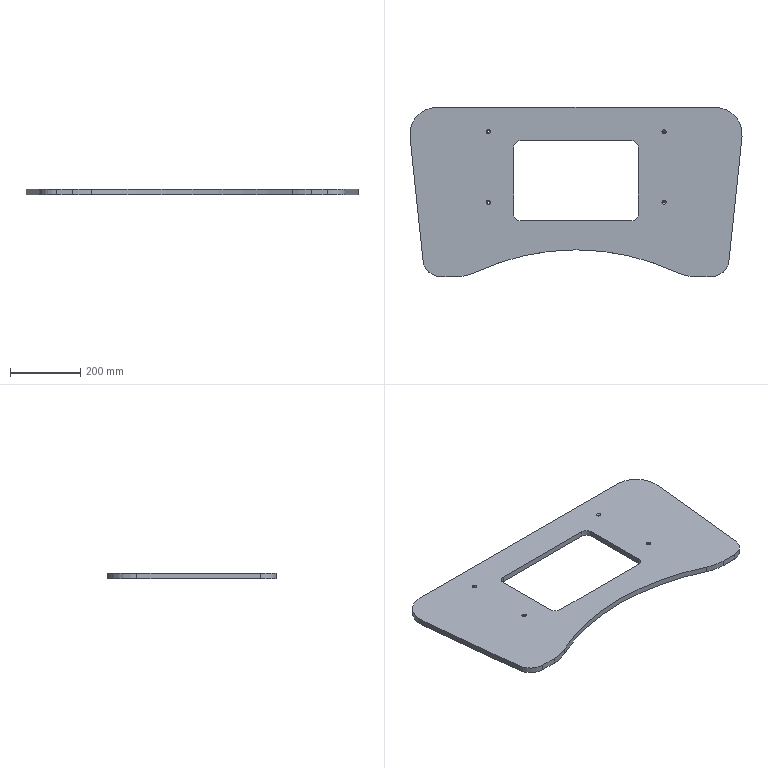Part | NX | features BREP 1 | 1 solid | 38 faces | box 948.321 x 482.727 x 15.875 mm | volume 5145279 mm3 | cylinder 19 | plane 11 | cone 8 | commonest cylinder face diameters 6.604 x8 38.1 x4 101.6 x2 152.4 x2 254 x2 1347 x1
STEP:
#1=CARTESIAN_POINT('',(-386.065,-482.727,0.));
#2=VERTEX_POINT('',#1);
#3=CARTESIAN_POINT('',(-340.836,-482.727,0.));
#4=VERTEX_POINT('',#3);
#5=CARTESIAN_POINT('',(-386.065,-482.727,0.));
#6=DIRECTION('',(1.,0.,0.));
#7=VECTOR('',#6,1000.);
#8=LINE('',#5,#7);
#9=EDGE_CURVE('',#2,#4,#8,.T.);
#10=ORIENTED_EDGE('',*,*,#9,.F.);
#11=CARTESIAN_POINT('',(-436.586,-437.244,0.));
#12=VERTEX_POINT('',#11);
#13=CARTESIAN_POINT('',(-386.065,-431.927,0.));
#14=DIRECTION('',(0.,0.,-1.));
#15=DIRECTION('',(0.,-1.,0.));
#16=AXIS2_PLACEMENT_3D('',#13,#14,#15);
#17=CIRCLE('',#16,50.8);
#18=EDGE_CURVE('',#2,#12,#17,.T.);
#19=ORIENTED_EDGE('',*,*,#18,.T.);
#20=CARTESIAN_POINT('',(-473.742,-84.175,0.));
#21=VERTEX_POINT('',#20);
#22=CARTESIAN_POINT('',(-473.742,-84.175,0.));
#23=DIRECTION('',(0.1047,-0.9945,0.));
#24=VECTOR('',#23,1000.);
#25=LINE('',#22,#24);
#26=EDGE_CURVE('',#21,#12,#25,.T.);
#27=ORIENTED_EDGE('',*,*,#26,.F.);
#28=CARTESIAN_POINT('',(-397.96,0.,0.));
#29=VERTEX_POINT('',#28);
#30=CARTESIAN_POINT('',(-397.96,-76.2,0.));
#31=DIRECTION('',(0.,0.,-1.));
#32=DIRECTION('',(-0.9945,-0.1047,0.));
#33=AXIS2_PLACEMENT_3D('',#30,#31,#32);
#34=CIRCLE('',#33,76.2);
#35=EDGE_CURVE('',#21,#29,#34,.T.);
#36=ORIENTED_EDGE('',*,*,#35,.T.);
#37=CARTESIAN_POINT('',(397.96,0.,0.));
#38=VERTEX_POINT('',#37);
#39=CARTESIAN_POINT('',(397.96,0.,0.));
#40=DIRECTION('',(-1.,0.,0.));
#41=VECTOR('',#40,1000.);
#42=LINE('',#39,#41);
#43=EDGE_CURVE('',#38,#29,#42,.T.);
#44=ORIENTED_EDGE('',*,*,#43,.F.);
#45=CARTESIAN_POINT('',(473.742,-84.175,0.));
#46=VERTEX_POINT('',#45);
#47=CARTESIAN_POINT('',(397.96,-76.2,0.));
#48=DIRECTION('',(0.,0.,-1.));
#49=DIRECTION('',(0.,1.,0.));
#50=AXIS2_PLACEMENT_3D('',#47,#48,#49);
#51=CIRCLE('',#50,76.2);
#52=EDGE_CURVE('',#38,#46,#51,.T.);
#53=ORIENTED_EDGE('',*,*,#52,.T.);
#54=CARTESIAN_POINT('',(436.586,-437.244,0.));
#55=VERTEX_POINT('',#54);
#56=CARTESIAN_POINT('',(436.586,-437.244,0.));
#57=DIRECTION('',(0.1047,0.9945,0.));
#58=VECTOR('',#57,1000.);
#59=LINE('',#56,#58);
#60=EDGE_CURVE('',#55,#46,#59,.T.);
#61=ORIENTED_EDGE('',*,*,#60,.F.);
#62=CARTESIAN_POINT('',(386.065,-482.727,0.));
#63=VERTEX_POINT('',#62);
#64=CARTESIAN_POINT('',(386.065,-431.927,0.));
#65=DIRECTION('',(0.,0.,-1.));
#66=DIRECTION('',(0.9945,-0.1047,0.));
#67=AXIS2_PLACEMENT_3D('',#64,#65,#66);
#68=CIRCLE('',#67,50.8);
#69=EDGE_CURVE('',#55,#63,#68,.T.);
#70=ORIENTED_EDGE('',*,*,#69,.T.);
#71=CARTESIAN_POINT('',(340.836,-482.727,0.));
#72=VERTEX_POINT('',#71);
#73=CARTESIAN_POINT('',(340.836,-482.727,0.));
#74=DIRECTION('',(1.,0.,0.));
#75=VECTOR('',#74,1000.);
#76=LINE('',#73,#75);
#77=EDGE_CURVE('',#72,#63,#76,.T.);
#78=ORIENTED_EDGE('',*,*,#77,.F.);
#79=CARTESIAN_POINT('',(286.753,-470.636,0.));
#80=VERTEX_POINT('',#79);
#81=CARTESIAN_POINT('',(340.836,-355.727,0.));
#82=DIRECTION('',(0.,0.,-1.));
#83=DIRECTION('',(0.,-1.,0.));
#84=AXIS2_PLACEMENT_3D('',#81,#82,#83);
#85=CIRCLE('',#84,127.);
#86=EDGE_CURVE('',#72,#80,#85,.T.);
#87=ORIENTED_EDGE('',*,*,#86,.T.);
#88=CARTESIAN_POINT('',(-286.753,-470.636,0.));
#89=VERTEX_POINT('',#88);
#90=CARTESIAN_POINT('',(0.,-1079.892,0.));
#91=DIRECTION('',(0.,0.,1.));
#92=DIRECTION('',(0.4259,0.9048,0.));
#93=AXIS2_PLACEMENT_3D('',#90,#91,#92);
#94=CIRCLE('',#93,673.365);
#95=EDGE_CURVE('',#80,#89,#94,.T.);
#96=ORIENTED_EDGE('',*,*,#95,.T.);
#97=CARTESIAN_POINT('',(-340.836,-355.727,0.));
#98=DIRECTION('',(0.,0.,-1.));
#99=DIRECTION('',(0.4259,-0.9048,0.));
#100=AXIS2_PLACEMENT_3D('',#97,#98,#99);
#101=CIRCLE('',#100,127.);
#102=EDGE_CURVE('',#89,#4,#101,.T.);
#103=ORIENTED_EDGE('',*,*,#102,.T.);
#104=EDGE_LOOP('',(#10,#19,#27,#36,#44,#53,#61,#70,#78,#87,#96,#103));
#105=FACE_BOUND('',#104,.T.);
#106=CARTESIAN_POINT('',(-246.888,-270.51,0.));
#107=VERTEX_POINT('',#106);
#108=CARTESIAN_POINT('',(-253.492,-270.51,0.));
#109=VERTEX_POINT('',#108);
#110=CARTESIAN_POINT('',(-250.19,-270.51,0.));
#111=DIRECTION('',(0.,0.,1.));
#112=DIRECTION('',(1.,0.,0.));
#113=AXIS2_PLACEMENT_3D('',#110,#111,#112);
#114=CIRCLE('',#113,3.302);
#115=EDGE_CURVE('',#107,#109,#114,.T.);
#116=ORIENTED_EDGE('',*,*,#115,.T.);
#117=CARTESIAN_POINT('',(-250.19,-270.51,0.));
#118=DIRECTION('',(0.,0.,1.));
#119=DIRECTION('',(-1.,0.,0.));
#120=AXIS2_PLACEMENT_3D('',#117,#118,#119);
#121=CIRCLE('',#120,3.302);
#122=EDGE_CURVE('',#109,#107,#121,.T.);
#123=ORIENTED_EDGE('',*,*,#122,.T.);
#124=EDGE_LOOP('',(#116,#123));
#125=FACE_BOUND('',#124,.T.);
#126=CARTESIAN_POINT('',(254.762,-69.85,0.));
#127=VERTEX_POINT('',#126);
#128=CARTESIAN_POINT('',(248.158,-69.85,0.));
#129=VERTEX_POINT('',#128);
#130=CARTESIAN_POINT('',(251.46,-69.85,0.));
#131=DIRECTION('',(0.,0.,1.));
#132=DIRECTION('',(1.,0.,0.));
#133=AXIS2_PLACEMENT_3D('',#130,#131,#132);
#134=CIRCLE('',#133,3.302);
#135=EDGE_CURVE('',#127,#129,#134,.T.);
#136=ORIENTED_EDGE('',*,*,#135,.T.);
#137=CARTESIAN_POINT('',(251.46,-69.85,0.));
#138=DIRECTION('',(0.,0.,1.));
#139=DIRECTION('',(-1.,0.,0.));
#140=AXIS2_PLACEMENT_3D('',#137,#138,#139);
#141=CIRCLE('',#140,3.302);
#142=EDGE_CURVE('',#129,#127,#141,.T.);
#143=ORIENTED_EDGE('',*,*,#142,.T.);
#144=EDGE_LOOP('',(#136,#143));
#145=FACE_BOUND('',#144,.T.);
#146=CARTESIAN_POINT('',(-177.8,-304.8,0.));
#147=VERTEX_POINT('',#146);
#148=CARTESIAN_POINT('',(-158.75,-323.85,0.));
#149=VERTEX_POINT('',#148);
#150=CARTESIAN_POINT('',(-158.75,-304.8,0.));
#151=DIRECTION('',(0.,0.,1.));
#152=DIRECTION('',(-1.,0.,0.));
#153=AXIS2_PLACEMENT_3D('',#150,#151,#152);
#154=CIRCLE('',#153,19.05);
#155=EDGE_CURVE('',#147,#149,#154,.T.);
#156=ORIENTED_EDGE('',*,*,#155,.T.);
#157=CARTESIAN_POINT('',(158.75,-323.85,0.));
#158=VERTEX_POINT('',#157);
#159=CARTESIAN_POINT('',(-158.75,-323.85,0.));
#160=DIRECTION('',(1.,0.,0.));
#161=VECTOR('',#160,1000.);
#162=LINE('',#159,#161);
#163=EDGE_CURVE('',#149,#158,#162,.T.);
#164=ORIENTED_EDGE('',*,*,#163,.T.);
#165=CARTESIAN_POINT('',(177.8,-304.8,0.));
#166=VERTEX_POINT('',#165);
#167=CARTESIAN_POINT('',(158.75,-304.8,0.));
#168=DIRECTION('',(0.,0.,1.));
#169=DIRECTION('',(0.,-1.,0.));
#170=AXIS2_PLACEMENT_3D('',#167,#168,#169);
#171=CIRCLE('',#170,19.05);
#172=EDGE_CURVE('',#158,#166,#171,.T.);
#173=ORIENTED_EDGE('',*,*,#172,.T.);
#174=CARTESIAN_POINT('',(177.8,-114.3,0.));
#175=VERTEX_POINT('',#174);
#176=CARTESIAN_POINT('',(177.8,-304.8,0.));
#177=DIRECTION('',(0.,1.,0.));
#178=VECTOR('',#177,1000.);
#179=LINE('',#176,#178);
#180=EDGE_CURVE('',#166,#175,#179,.T.);
#181=ORIENTED_EDGE('',*,*,#180,.T.);
#182=CARTESIAN_POINT('',(158.75,-95.25,0.));
#183=VERTEX_POINT('',#182);
#184=CARTESIAN_POINT('',(158.75,-114.3,0.));
#185=DIRECTION('',(0.,0.,1.));
#186=DIRECTION('',(1.,0.,0.));
#187=AXIS2_PLACEMENT_3D('',#184,#185,#186);
#188=CIRCLE('',#187,19.05);
#189=EDGE_CURVE('',#175,#183,#188,.T.);
#190=ORIENTED_EDGE('',*,*,#189,.T.);
#191=CARTESIAN_POINT('',(-158.75,-95.25,0.));
#192=VERTEX_POINT('',#191);
#193=CARTESIAN_POINT('',(158.75,-95.25,0.));
#194=DIRECTION('',(-1.,0.,0.));
#195=VECTOR('',#194,1000.);
#196=LINE('',#193,#195);
#197=EDGE_CURVE('',#183,#192,#196,.T.);
#198=ORIENTED_EDGE('',*,*,#197,.T.);
#199=CARTESIAN_POINT('',(-177.8,-114.3,0.));
#200=VERTEX_POINT('',#199);
#201=CARTESIAN_POINT('',(-158.75,-114.3,0.));
#202=DIRECTION('',(0.,0.,1.));
#203=DIRECTION('',(0.,1.,0.));
#204=AXIS2_PLACEMENT_3D('',#201,#202,#203);
#205=CIRCLE('',#204,19.05);
#206=EDGE_CURVE('',#192,#200,#205,.T.);
#207=ORIENTED_EDGE('',*,*,#206,.T.);
#208=CARTESIAN_POINT('',(-177.8,-114.3,0.));
#209=DIRECTION('',(0.,-1.,0.));
#210=VECTOR('',#209,1000.);
#211=LINE('',#208,#210);
#212=EDGE_CURVE('',#200,#147,#211,.T.);
#213=ORIENTED_EDGE('',*,*,#212,.T.);
#214=EDGE_LOOP('',(#156,#164,#173,#181,#190,#198,#207,#213));
#215=FACE_BOUND('',#214,.T.);
#216=CARTESIAN_POINT('',(254.762,-270.51,0.));
#217=VERTEX_POINT('',#216);
#218=CARTESIAN_POINT('',(248.158,-270.51,0.));
#219=VERTEX_POINT('',#218);
#220=CARTESIAN_POINT('',(251.46,-270.51,0.));
#221=DIRECTION('',(0.,0.,1.));
#222=DIRECTION('',(1.,0.,0.));
#223=AXIS2_PLACEMENT_3D('',#220,#221,#222);
#224=CIRCLE('',#223,3.302);
#225=EDGE_CURVE('',#217,#219,#224,.T.);
#226=ORIENTED_EDGE('',*,*,#225,.T.);
#227=CARTESIAN_POINT('',(251.46,-270.51,0.));
#228=DIRECTION('',(0.,0.,1.));
#229=DIRECTION('',(-1.,0.,0.));
#230=AXIS2_PLACEMENT_3D('',#227,#228,#229);
#231=CIRCLE('',#230,3.302);
#232=EDGE_CURVE('',#219,#217,#231,.T.);
#233=ORIENTED_EDGE('',*,*,#232,.T.);
#234=EDGE_LOOP('',(#226,#233));
#235=FACE_BOUND('',#234,.T.);
#236=CARTESIAN_POINT('',(-246.888,-69.85,0.));
#237=VERTEX_POINT('',#236);
#238=CARTESIAN_POINT('',(-253.492,-69.85,0.));
#239=VERTEX_POINT('',#238);
#240=CARTESIAN_POINT('',(-250.19,-69.85,0.));
#241=DIRECTION('',(0.,0.,1.));
#242=DIRECTION('',(1.,0.,0.));
#243=AXIS2_PLACEMENT_3D('',#240,#241,#242);
#244=CIRCLE('',#243,3.302);
#245=EDGE_CURVE('',#237,#239,#244,.T.);
#246=ORIENTED_EDGE('',*,*,#245,.T.);
#247=CARTESIAN_POINT('',(-250.19,-69.85,0.));
#248=DIRECTION('',(0.,0.,1.));
#249=DIRECTION('',(-1.,0.,0.));
#250=AXIS2_PLACEMENT_3D('',#247,#248,#249);
#251=CIRCLE('',#250,3.302);
#252=EDGE_CURVE('',#239,#237,#251,.T.);
#253=ORIENTED_EDGE('',*,*,#252,.T.);
#254=EDGE_LOOP('',(#246,#253));
#255=FACE_BOUND('',#254,.T.);
#256=CARTESIAN_POINT('',(0.,0.,0.));
#257=DIRECTION('',(0.,0.,1.));
#258=DIRECTION('',(1.,0.,0.));
#259=AXIS2_PLACEMENT_3D('',#256,#257,#258);
#260=PLANE('',#259);
#261=ADVANCED_FACE('',(#105,#125,#145,#215,#235,#255),#260,.F.);
#262=CARTESIAN_POINT('',(248.158,-270.51,12.734));
#263=VERTEX_POINT('',#262);
#264=CARTESIAN_POINT('',(248.158,-270.51,0.));
#265=DIRECTION('',(0.,0.,1.));
#266=VECTOR('',#265,1000.);
#267=LINE('',#264,#266);
#268=EDGE_CURVE('',#219,#263,#267,.T.);
#269=ORIENTED_EDGE('',*,*,#268,.T.);
#270=CARTESIAN_POINT('',(254.762,-270.51,12.734));
#271=VERTEX_POINT('',#270);
#272=CARTESIAN_POINT('',(251.46,-270.51,12.734));
#273=DIRECTION('',(0.,0.,1.));
#274=DIRECTION('',(-1.,0.,0.));
#275=AXIS2_PLACEMENT_3D('',#272,#273,#274);
#276=CIRCLE('',#275,3.302);
#277=EDGE_CURVE('',#263,#271,#276,.T.);
#278=ORIENTED_EDGE('',*,*,#277,.T.);
#279=CARTESIAN_POINT('',(254.762,-270.51,0.));
#280=DIRECTION('',(0.,0.,1.));
#281=VECTOR('',#280,1000.);
#282=LINE('',#279,#281);
#283=EDGE_CURVE('',#217,#271,#282,.T.);
#284=ORIENTED_EDGE('',*,*,#283,.F.);
#285=ORIENTED_EDGE('',*,*,#232,.F.);
#286=EDGE_LOOP('',(#269,#278,#284,#285));
#287=FACE_BOUND('',#286,.T.);
#288=CARTESIAN_POINT('',(251.46,-270.51,-4.128));
#289=DIRECTION('',(0.,0.,1.));
#290=DIRECTION('',(-1.,0.,0.));
#291=AXIS2_PLACEMENT_3D('',#288,#289,#290);
#292=CYLINDRICAL_SURFACE('',#291,3.302);
#293=ADVANCED_FACE('',(#287),#292,.F.);
#294=ORIENTED_EDGE('',*,*,#283,.T.);
#295=CARTESIAN_POINT('',(251.46,-270.51,12.734));
#296=DIRECTION('',(0.,0.,-1.));
#297=DIRECTION('',(-1.,0.,0.));
#298=AXIS2_PLACEMENT_3D('',#295,#296,#297);
#299=CIRCLE('',#298,3.302);
#300=EDGE_CURVE('',#263,#271,#299,.T.);
#301=ORIENTED_EDGE('',*,*,#300,.F.);
#302=ORIENTED_EDGE('',*,*,#268,.F.);
#303=ORIENTED_EDGE('',*,*,#225,.F.);
#304=EDGE_LOOP('',(#294,#301,#302,#303));
#305=FACE_BOUND('',#304,.T.);
#306=CARTESIAN_POINT('',(251.46,-270.51,-4.128));
#307=DIRECTION('',(0.,0.,1.));
#308=DIRECTION('',(-1.,0.,0.));
#309=AXIS2_PLACEMENT_3D('',#306,#307,#308);
#310=CYLINDRICAL_SURFACE('',#309,3.302);
#311=ADVANCED_FACE('',(#305),#310,.F.);
#312=CARTESIAN_POINT('',(245.428,-270.51,15.875));
#313=VERTEX_POINT('',#312);
#314=CARTESIAN_POINT('',(248.158,-270.51,12.734));
#315=DIRECTION('',(-0.6561,0.,0.7547));
#316=VECTOR('',#315,1000.);
#317=LINE('',#314,#316);
#318=EDGE_CURVE('',#263,#313,#317,.T.);
#319=ORIENTED_EDGE('',*,*,#318,.F.);
#320=ORIENTED_EDGE('',*,*,#300,.T.);
#321=CARTESIAN_POINT('',(257.493,-270.51,15.875));
#322=VERTEX_POINT('',#321);
#323=CARTESIAN_POINT('',(254.762,-270.51,12.734));
#324=DIRECTION('',(0.6561,0.,0.7547));
#325=VECTOR('',#324,1000.);
#326=LINE('',#323,#325);
#327=EDGE_CURVE('',#271,#322,#326,.T.);
#328=ORIENTED_EDGE('',*,*,#327,.T.);
#329=CARTESIAN_POINT('',(251.46,-270.51,15.875));
#330=DIRECTION('',(0.,0.,1.));
#331=DIRECTION('',(1.,0.,0.));
#332=AXIS2_PLACEMENT_3D('',#329,#330,#331);
#333=CIRCLE('',#332,6.032);
#334=EDGE_CURVE('',#322,#313,#333,.T.);
#335=ORIENTED_EDGE('',*,*,#334,.T.);
#336=EDGE_LOOP('',(#319,#320,#328,#335));
#337=FACE_BOUND('',#336,.T.);
#338=CARTESIAN_POINT('',(251.46,-270.51,14.304));
#339=DIRECTION('',(0.,0.,1.));
#340=DIRECTION('',(-1.,0.,0.));
#341=AXIS2_PLACEMENT_3D('',#338,#339,#340);
#342=CONICAL_SURFACE('',#341,4.667,0.7156);
#343=ADVANCED_FACE('',(#337),#342,.F.);
#344=CARTESIAN_POINT('',(286.753,-470.636,15.875));
#345=VERTEX_POINT('',#344);
#346=CARTESIAN_POINT('',(-286.753,-470.636,15.875));
#347=VERTEX_POINT('',#346);
#348=CARTESIAN_POINT('',(0.,-1079.892,15.875));
#349=DIRECTION('',(0.,0.,1.));
#350=DIRECTION('',(0.4259,0.9048,0.));
#351=AXIS2_PLACEMENT_3D('',#348,#349,#350);
#352=CIRCLE('',#351,673.365);
#353=EDGE_CURVE('',#345,#347,#352,.T.);
#354=ORIENTED_EDGE('',*,*,#353,.F.);
#355=CARTESIAN_POINT('',(340.836,-482.727,15.875));
#356=VERTEX_POINT('',#355);
#357=CARTESIAN_POINT('',(340.836,-355.727,15.875));
#358=DIRECTION('',(0.,0.,1.));
#359=DIRECTION('',(-0.4259,-0.9048,0.));
#360=AXIS2_PLACEMENT_3D('',#357,#358,#359);
#361=CIRCLE('',#360,127.);
#362=EDGE_CURVE('',#345,#356,#361,.T.);
#363=ORIENTED_EDGE('',*,*,#362,.T.);
#364=CARTESIAN_POINT('',(386.065,-482.727,15.875));
#365=VERTEX_POINT('',#364);
#366=CARTESIAN_POINT('',(340.836,-482.727,15.875));
#367=DIRECTION('',(1.,0.,0.));
#368=VECTOR('',#367,1000.);
#369=LINE('',#366,#368);
#370=EDGE_CURVE('',#356,#365,#369,.T.);
#371=ORIENTED_EDGE('',*,*,#370,.T.);
#372=CARTESIAN_POINT('',(436.586,-437.244,15.875));
#373=VERTEX_POINT('',#372);
#374=CARTESIAN_POINT('',(386.065,-431.927,15.875));
#375=DIRECTION('',(0.,0.,1.));
#376=DIRECTION('',(0.,-1.,0.));
#377=AXIS2_PLACEMENT_3D('',#374,#375,#376);
#378=CIRCLE('',#377,50.8);
#379=EDGE_CURVE('',#365,#373,#378,.T.);
#380=ORIENTED_EDGE('',*,*,#379,.T.);
#381=CARTESIAN_POINT('',(473.742,-84.175,15.875));
#382=VERTEX_POINT('',#381);
#383=CARTESIAN_POINT('',(436.586,-437.244,15.875));
#384=DIRECTION('',(0.1047,0.9945,0.));
#385=VECTOR('',#384,1000.);
#386=LINE('',#383,#385);
#387=EDGE_CURVE('',#373,#382,#386,.T.);
#388=ORIENTED_EDGE('',*,*,#387,.T.);
#389=CARTESIAN_POINT('',(397.96,0.,15.875));
#390=VERTEX_POINT('',#389);
#391=CARTESIAN_POINT('',(397.96,-76.2,15.875));
#392=DIRECTION('',(0.,0.,1.));
#393=DIRECTION('',(0.9945,-0.1047,0.));
#394=AXIS2_PLACEMENT_3D('',#391,#392,#393);
#395=CIRCLE('',#394,76.2);
#396=EDGE_CURVE('',#382,#390,#395,.T.);
#397=ORIENTED_EDGE('',*,*,#396,.T.);
#398=CARTESIAN_POINT('',(-397.96,0.,15.875));
#399=VERTEX_POINT('',#398);
#400=CARTESIAN_POINT('',(397.96,0.,15.875));
#401=DIRECTION('',(-1.,0.,0.));
#402=VECTOR('',#401,1000.);
#403=LINE('',#400,#402);
#404=EDGE_CURVE('',#390,#399,#403,.T.);
#405=ORIENTED_EDGE('',*,*,#404,.T.);
#406=CARTESIAN_POINT('',(-473.742,-84.175,15.875));
#407=VERTEX_POINT('',#406);
#408=CARTESIAN_POINT('',(-397.96,-76.2,15.875));
#409=DIRECTION('',(0.,0.,1.));
#410=DIRECTION('',(0.,1.,0.));
#411=AXIS2_PLACEMENT_3D('',#408,#409,#410);
#412=CIRCLE('',#411,76.2);
#413=EDGE_CURVE('',#399,#407,#412,.T.);
#414=ORIENTED_EDGE('',*,*,#413,.T.);
#415=CARTESIAN_POINT('',(-436.586,-437.244,15.875));
#416=VERTEX_POINT('',#415);
#417=CARTESIAN_POINT('',(-473.742,-84.175,15.875));
#418=DIRECTION('',(0.1047,-0.9945,0.));
#419=VECTOR('',#418,1000.);
#420=LINE('',#417,#419);
#421=EDGE_CURVE('',#407,#416,#420,.T.);
#422=ORIENTED_EDGE('',*,*,#421,.T.);
#423=CARTESIAN_POINT('',(-386.065,-482.727,15.875));
#424=VERTEX_POINT('',#423);
#425=CARTESIAN_POINT('',(-386.065,-431.927,15.875));
#426=DIRECTION('',(0.,0.,1.));
#427=DIRECTION('',(-0.9945,-0.1047,0.));
#428=AXIS2_PLACEMENT_3D('',#425,#426,#427);
#429=CIRCLE('',#428,50.8);
#430=EDGE_CURVE('',#416,#424,#429,.T.);
#431=ORIENTED_EDGE('',*,*,#430,.T.);
#432=CARTESIAN_POINT('',(-340.836,-482.727,15.875));
#433=VERTEX_POINT('',#432);
#434=CARTESIAN_POINT('',(-386.065,-482.727,15.875));
#435=DIRECTION('',(1.,0.,0.));
#436=VECTOR('',#435,1000.);
#437=LINE('',#434,#436);
#438=EDGE_CURVE('',#424,#433,#437,.T.);
#439=ORIENTED_EDGE('',*,*,#438,.T.);
#440=CARTESIAN_POINT('',(-340.836,-355.727,15.875));
#441=DIRECTION('',(0.,0.,1.));
#442=DIRECTION('',(0.,-1.,0.));
#443=AXIS2_PLACEMENT_3D('',#440,#441,#442);
#444=CIRCLE('',#443,127.);
#445=EDGE_CURVE('',#433,#347,#444,.T.);
#446=ORIENTED_EDGE('',*,*,#445,.T.);
#447=EDGE_LOOP('',(#354,#363,#371,#380,#388,#397,#405,#414,#422,#431,#439,#446));
#448=FACE_BOUND('',#447,.T.);
#449=CARTESIAN_POINT('',(-244.157,-270.51,15.875));
#450=VERTEX_POINT('',#449);
#451=CARTESIAN_POINT('',(-256.223,-270.51,15.875));
#452=VERTEX_POINT('',#451);
#453=CARTESIAN_POINT('',(-250.19,-270.51,15.875));
#454=DIRECTION('',(0.,0.,1.));
#455=DIRECTION('',(1.,0.,0.));
#456=AXIS2_PLACEMENT_3D('',#453,#454,#455);
#457=CIRCLE('',#456,6.032);
#458=EDGE_CURVE('',#450,#452,#457,.T.);
#459=ORIENTED_EDGE('',*,*,#458,.F.);
#460=CARTESIAN_POINT('',(-250.19,-270.51,15.875));
#461=DIRECTION('',(0.,0.,1.));
#462=DIRECTION('',(-1.,0.,0.));
#463=AXIS2_PLACEMENT_3D('',#460,#461,#462);
#464=CIRCLE('',#463,6.032);
#465=EDGE_CURVE('',#452,#450,#464,.T.);
#466=ORIENTED_EDGE('',*,*,#465,.F.);
#467=EDGE_LOOP('',(#459,#466));
#468=FACE_BOUND('',#467,.T.);
#469=CARTESIAN_POINT('',(257.493,-69.85,15.875));
#470=VERTEX_POINT('',#469);
#471=CARTESIAN_POINT('',(245.428,-69.85,15.875));
#472=VERTEX_POINT('',#471);
#473=CARTESIAN_POINT('',(251.46,-69.85,15.875));
#474=DIRECTION('',(0.,0.,1.));
#475=DIRECTION('',(1.,0.,0.));
#476=AXIS2_PLACEMENT_3D('',#473,#474,#475);
#477=CIRCLE('',#476,6.032);
#478=EDGE_CURVE('',#470,#472,#477,.T.);
#479=ORIENTED_EDGE('',*,*,#478,.F.);
#480=CARTESIAN_POINT('',(251.46,-69.85,15.875));
#481=DIRECTION('',(0.,0.,1.));
#482=DIRECTION('',(-1.,0.,0.));
#483=AXIS2_PLACEMENT_3D('',#480,#481,#482);
#484=CIRCLE('',#483,6.032);
#485=EDGE_CURVE('',#472,#470,#484,.T.);
#486=ORIENTED_EDGE('',*,*,#485,.F.);
#487=EDGE_LOOP('',(#479,#486));
#488=FACE_BOUND('',#487,.T.);
#489=CARTESIAN_POINT('',(158.75,-95.25,15.875));
#490=VERTEX_POINT('',#489);
#491=CARTESIAN_POINT('',(177.8,-114.3,15.875));
#492=VERTEX_POINT('',#491);
#493=CARTESIAN_POINT('',(158.75,-114.3,15.875));
#494=DIRECTION('',(0.,0.,-1.));
#495=DIRECTION('',(0.,1.,0.));
#496=AXIS2_PLACEMENT_3D('',#493,#494,#495);
#497=CIRCLE('',#496,19.05);
#498=EDGE_CURVE('',#490,#492,#497,.T.);
#499=ORIENTED_EDGE('',*,*,#498,.T.);
#500=CARTESIAN_POINT('',(177.8,-304.8,15.875));
#501=VERTEX_POINT('',#500);
#502=CARTESIAN_POINT('',(177.8,-304.8,15.875));
#503=DIRECTION('',(0.,1.,0.));
#504=VECTOR('',#503,1000.);
#505=LINE('',#502,#504);
#506=EDGE_CURVE('',#501,#492,#505,.T.);
#507=ORIENTED_EDGE('',*,*,#506,.F.);
#508=CARTESIAN_POINT('',(158.75,-323.85,15.875));
#509=VERTEX_POINT('',#508);
#510=CARTESIAN_POINT('',(158.75,-304.8,15.875));
#511=DIRECTION('',(0.,0.,-1.));
#512=DIRECTION('',(1.,0.,0.));
#513=AXIS2_PLACEMENT_3D('',#510,#511,#512);
#514=CIRCLE('',#513,19.05);
#515=EDGE_CURVE('',#501,#509,#514,.T.);
#516=ORIENTED_EDGE('',*,*,#515,.T.);
#517=CARTESIAN_POINT('',(-158.75,-323.85,15.875));
#518=VERTEX_POINT('',#517);
#519=CARTESIAN_POINT('',(-158.75,-323.85,15.875));
#520=DIRECTION('',(1.,0.,0.));
#521=VECTOR('',#520,1000.);
#522=LINE('',#519,#521);
#523=EDGE_CURVE('',#518,#509,#522,.T.);
#524=ORIENTED_EDGE('',*,*,#523,.F.);
#525=CARTESIAN_POINT('',(-177.8,-304.8,15.875));
#526=VERTEX_POINT('',#525);
#527=CARTESIAN_POINT('',(-158.75,-304.8,15.875));
#528=DIRECTION('',(0.,0.,-1.));
#529=DIRECTION('',(0.,-1.,0.));
#530=AXIS2_PLACEMENT_3D('',#527,#528,#529);
#531=CIRCLE('',#530,19.05);
#532=EDGE_CURVE('',#518,#526,#531,.T.);
#533=ORIENTED_EDGE('',*,*,#532,.T.);
#534=CARTESIAN_POINT('',(-177.8,-114.3,15.875));
#535=VERTEX_POINT('',#534);
#536=CARTESIAN_POINT('',(-177.8,-114.3,15.875));
#537=DIRECTION('',(0.,-1.,0.));
#538=VECTOR('',#537,1000.);
#539=LINE('',#536,#538);
#540=EDGE_CURVE('',#535,#526,#539,.T.);
#541=ORIENTED_EDGE('',*,*,#540,.F.);
#542=CARTESIAN_POINT('',(-158.75,-95.25,15.875));
#543=VERTEX_POINT('',#542);
#544=CARTESIAN_POINT('',(-158.75,-114.3,15.875));
#545=DIRECTION('',(0.,0.,-1.));
#546=DIRECTION('',(-1.,0.,0.));
#547=AXIS2_PLACEMENT_3D('',#544,#545,#546);
#548=CIRCLE('',#547,19.05);
#549=EDGE_CURVE('',#535,#543,#548,.T.);
#550=ORIENTED_EDGE('',*,*,#549,.T.);
#551=CARTESIAN_POINT('',(158.75,-95.25,15.875));
#552=DIRECTION('',(-1.,0.,0.));
#553=VECTOR('',#552,1000.);
#554=LINE('',#551,#553);
#555=EDGE_CURVE('',#490,#543,#554,.T.);
#556=ORIENTED_EDGE('',*,*,#555,.F.);
#557=EDGE_LOOP('',(#499,#507,#516,#524,#533,#541,#550,#556));
#558=FACE_BOUND('',#557,.T.);
#559=ORIENTED_EDGE('',*,*,#334,.F.);
#560=CARTESIAN_POINT('',(251.46,-270.51,15.875));
#561=DIRECTION('',(0.,0.,1.));
#562=DIRECTION('',(-1.,0.,0.));
#563=AXIS2_PLACEMENT_3D('',#560,#561,#562);
#564=CIRCLE('',#563,6.032);
#565=EDGE_CURVE('',#313,#322,#564,.T.);
#566=ORIENTED_EDGE('',*,*,#565,.F.);
#567=EDGE_LOOP('',(#559,#566));
#568=FACE_BOUND('',#567,.T.);
#569=CARTESIAN_POINT('',(-244.157,-69.85,15.875));
#570=VERTEX_POINT('',#569);
#571=CARTESIAN_POINT('',(-256.223,-69.85,15.875));
#572=VERTEX_POINT('',#571);
#573=CARTESIAN_POINT('',(-250.19,-69.85,15.875));
#574=DIRECTION('',(0.,0.,1.));
#575=DIRECTION('',(1.,0.,0.));
#576=AXIS2_PLACEMENT_3D('',#573,#574,#575);
#577=CIRCLE('',#576,6.032);
#578=EDGE_CURVE('',#570,#572,#577,.T.);
#579=ORIENTED_EDGE('',*,*,#578,.F.);
#580=CARTESIAN_POINT('',(-250.19,-69.85,15.875));
#581=DIRECTION('',(0.,0.,1.));
#582=DIRECTION('',(-1.,0.,0.));
#583=AXIS2_PLACEMENT_3D('',#580,#581,#582);
#584=CIRCLE('',#583,6.032);
#585=EDGE_CURVE('',#572,#570,#584,.T.);
#586=ORIENTED_EDGE('',*,*,#585,.F.);
#587=EDGE_LOOP('',(#579,#586));
#588=FACE_BOUND('',#587,.T.);
#589=CARTESIAN_POINT('',(0.,0.,15.875));
#590=DIRECTION('',(0.,0.,1.));
#591=DIRECTION('',(1.,0.,0.));
#592=AXIS2_PLACEMENT_3D('',#589,#590,#591);
#593=PLANE('',#592);
#594=ADVANCED_FACE('',(#448,#468,#488,#558,#568,#588),#593,.T.);
#595=ORIENTED_EDGE('',*,*,#327,.F.);
#596=ORIENTED_EDGE('',*,*,#277,.F.);
#597=ORIENTED_EDGE('',*,*,#318,.T.);
#598=ORIENTED_EDGE('',*,*,#565,.T.);
#599=EDGE_LOOP('',(#595,#596,#597,#598));
#600=FACE_BOUND('',#599,.T.);
#601=CARTESIAN_POINT('',(251.46,-270.51,14.304));
#602=DIRECTION('',(0.,0.,1.));
#603=DIRECTION('',(-1.,0.,0.));
#604=AXIS2_PLACEMENT_3D('',#601,#602,#603);
#605=CONICAL_SURFACE('',#604,4.667,0.7156);
#606=ADVANCED_FACE('',(#600),#605,.F.);
#607=CARTESIAN_POINT('',(-246.888,-270.51,12.734));
#608=VERTEX_POINT('',#607);
#609=CARTESIAN_POINT('',(-246.888,-270.51,12.734));
#610=DIRECTION('',(0.6561,0.,0.7547));
#611=VECTOR('',#610,1000.);
#612=LINE('',#609,#611);
#613=EDGE_CURVE('',#450,#608,#612,.F.);
#614=ORIENTED_EDGE('',*,*,#613,.T.);
#615=CARTESIAN_POINT('',(-253.492,-270.51,12.734));
#616=VERTEX_POINT('',#615);
#617=CARTESIAN_POINT('',(-250.19,-270.51,12.734));
#618=DIRECTION('',(0.,0.,1.));
#619=DIRECTION('',(-1.,0.,0.));
#620=AXIS2_PLACEMENT_3D('',#617,#618,#619);
#621=CIRCLE('',#620,3.302);
#622=EDGE_CURVE('',#616,#608,#621,.T.);
#623=ORIENTED_EDGE('',*,*,#622,.F.);
#624=CARTESIAN_POINT('',(-253.492,-270.51,12.734));
#625=DIRECTION('',(-0.6561,0.,0.7547));
#626=VECTOR('',#625,1000.);
#627=LINE('',#624,#626);
#628=EDGE_CURVE('',#452,#616,#627,.F.);
#629=ORIENTED_EDGE('',*,*,#628,.F.);
#630=ORIENTED_EDGE('',*,*,#465,.T.);
#631=EDGE_LOOP('',(#614,#623,#629,#630));
#632=FACE_BOUND('',#631,.T.);
#633=CARTESIAN_POINT('',(-250.19,-270.51,14.304));
#634=DIRECTION('',(0.,0.,1.));
#635=DIRECTION('',(-1.,0.,0.));
#636=AXIS2_PLACEMENT_3D('',#633,#634,#635);
#637=CONICAL_SURFACE('',#636,4.667,0.7156);
#638=ADVANCED_FACE('',(#632),#637,.F.);
#639=ORIENTED_EDGE('',*,*,#628,.T.);
#640=CARTESIAN_POINT('',(-250.19,-270.51,12.734));
#641=DIRECTION('',(0.,0.,-1.));
#642=DIRECTION('',(-1.,0.,0.));
#643=AXIS2_PLACEMENT_3D('',#640,#641,#642);
#644=CIRCLE('',#643,3.302);
#645=EDGE_CURVE('',#616,#608,#644,.T.);
#646=ORIENTED_EDGE('',*,*,#645,.T.);
#647=ORIENTED_EDGE('',*,*,#613,.F.);
#648=ORIENTED_EDGE('',*,*,#458,.T.);
#649=EDGE_LOOP('',(#639,#646,#647,#648));
#650=FACE_BOUND('',#649,.T.);
#651=CARTESIAN_POINT('',(-250.19,-270.51,14.304));
#652=DIRECTION('',(0.,0.,1.));
#653=DIRECTION('',(-1.,0.,0.));
#654=AXIS2_PLACEMENT_3D('',#651,#652,#653);
#655=CONICAL_SURFACE('',#654,4.667,0.7156);
#656=ADVANCED_FACE('',(#650),#655,.F.);
#657=CARTESIAN_POINT('',(-246.888,-270.51,0.));
#658=DIRECTION('',(0.,0.,1.));
#659=VECTOR('',#658,1000.);
#660=LINE('',#657,#659);
#661=EDGE_CURVE('',#608,#107,#660,.F.);
#662=ORIENTED_EDGE('',*,*,#661,.F.);
#663=ORIENTED_EDGE('',*,*,#645,.F.);
#664=CARTESIAN_POINT('',(-253.492,-270.51,0.));
#665=DIRECTION('',(0.,0.,1.));
#666=VECTOR('',#665,1000.);
#667=LINE('',#664,#666);
#668=EDGE_CURVE('',#616,#109,#667,.F.);
#669=ORIENTED_EDGE('',*,*,#668,.T.);
#670=ORIENTED_EDGE('',*,*,#115,.F.);
#671=EDGE_LOOP('',(#662,#663,#669,#670));
#672=FACE_BOUND('',#671,.T.);
#673=CARTESIAN_POINT('',(-250.19,-270.51,-4.128));
#674=DIRECTION('',(0.,0.,1.));
#675=DIRECTION('',(-1.,0.,0.));
#676=AXIS2_PLACEMENT_3D('',#673,#674,#675);
#677=CYLINDRICAL_SURFACE('',#676,3.302);
#678=ADVANCED_FACE('',(#672),#677,.F.);
#679=ORIENTED_EDGE('',*,*,#668,.F.);
#680=ORIENTED_EDGE('',*,*,#622,.T.);
#681=ORIENTED_EDGE('',*,*,#661,.T.);
#682=ORIENTED_EDGE('',*,*,#122,.F.);
#683=EDGE_LOOP('',(#679,#680,#681,#682));
#684=FACE_BOUND('',#683,.T.);
#685=CARTESIAN_POINT('',(-250.19,-270.51,-4.128));
#686=DIRECTION('',(0.,0.,1.));
#687=DIRECTION('',(-1.,0.,0.));
#688=AXIS2_PLACEMENT_3D('',#685,#686,#687);
#689=CYLINDRICAL_SURFACE('',#688,3.302);
#690=ADVANCED_FACE('',(#684),#689,.F.);
#691=CARTESIAN_POINT('',(254.762,-69.85,12.734));
#692=VERTEX_POINT('',#691);
#693=CARTESIAN_POINT('',(254.762,-69.85,12.734));
#694=DIRECTION('',(0.6561,0.,0.7547));
#695=VECTOR('',#694,1000.);
#696=LINE('',#693,#695);
#697=EDGE_CURVE('',#470,#692,#696,.F.);
#698=ORIENTED_EDGE('',*,*,#697,.T.);
#699=CARTESIAN_POINT('',(248.158,-69.85,12.734));
#700=VERTEX_POINT('',#699);
#701=CARTESIAN_POINT('',(251.46,-69.85,12.734));
#702=DIRECTION('',(0.,0.,1.));
#703=DIRECTION('',(-1.,0.,0.));
#704=AXIS2_PLACEMENT_3D('',#701,#702,#703);
#705=CIRCLE('',#704,3.302);
#706=EDGE_CURVE('',#700,#692,#705,.T.);
#707=ORIENTED_EDGE('',*,*,#706,.F.);
#708=CARTESIAN_POINT('',(248.158,-69.85,12.734));
#709=DIRECTION('',(-0.6561,0.,0.7547));
#710=VECTOR('',#709,1000.);
#711=LINE('',#708,#710);
#712=EDGE_CURVE('',#472,#700,#711,.F.);
#713=ORIENTED_EDGE('',*,*,#712,.F.);
#714=ORIENTED_EDGE('',*,*,#485,.T.);
#715=EDGE_LOOP('',(#698,#707,#713,#714));
#716=FACE_BOUND('',#715,.T.);
#717=CARTESIAN_POINT('',(251.46,-69.85,14.304));
#718=DIRECTION('',(0.,0.,1.));
#719=DIRECTION('',(-1.,0.,0.));
#720=AXIS2_PLACEMENT_3D('',#717,#718,#719);
#721=CONICAL_SURFACE('',#720,4.667,0.7156);
#722=ADVANCED_FACE('',(#716),#721,.F.);
#723=ORIENTED_EDGE('',*,*,#712,.T.);
#724=CARTESIAN_POINT('',(251.46,-69.85,12.734));
#725=DIRECTION('',(0.,0.,-1.));
#726=DIRECTION('',(-1.,0.,0.));
#727=AXIS2_PLACEMENT_3D('',#724,#725,#726);
#728=CIRCLE('',#727,3.302);
#729=EDGE_CURVE('',#700,#692,#728,.T.);
#730=ORIENTED_EDGE('',*,*,#729,.T.);
#731=ORIENTED_EDGE('',*,*,#697,.F.);
#732=ORIENTED_EDGE('',*,*,#478,.T.);
#733=EDGE_LOOP('',(#723,#730,#731,#732));
#734=FACE_BOUND('',#733,.T.);
#735=CARTESIAN_POINT('',(251.46,-69.85,14.304));
#736=DIRECTION('',(0.,0.,1.));
#737=DIRECTION('',(-1.,0.,0.));
#738=AXIS2_PLACEMENT_3D('',#735,#736,#737);
#739=CONICAL_SURFACE('',#738,4.667,0.7156);
#740=ADVANCED_FACE('',(#734),#739,.F.);
#741=CARTESIAN_POINT('',(254.762,-69.85,0.));
#742=DIRECTION('',(0.,0.,1.));
#743=VECTOR('',#742,1000.);
#744=LINE('',#741,#743);
#745=EDGE_CURVE('',#692,#127,#744,.F.);
#746=ORIENTED_EDGE('',*,*,#745,.F.);
#747=ORIENTED_EDGE('',*,*,#729,.F.);
#748=CARTESIAN_POINT('',(248.158,-69.85,0.));
#749=DIRECTION('',(0.,0.,1.));
#750=VECTOR('',#749,1000.);
#751=LINE('',#748,#750);
#752=EDGE_CURVE('',#700,#129,#751,.F.);
#753=ORIENTED_EDGE('',*,*,#752,.T.);
#754=ORIENTED_EDGE('',*,*,#135,.F.);
#755=EDGE_LOOP('',(#746,#747,#753,#754));
#756=FACE_BOUND('',#755,.T.);
#757=CARTESIAN_POINT('',(251.46,-69.85,-4.128));
#758=DIRECTION('',(0.,0.,1.));
#759=DIRECTION('',(-1.,0.,0.));
#760=AXIS2_PLACEMENT_3D('',#757,#758,#759);
#761=CYLINDRICAL_SURFACE('',#760,3.302);
#762=ADVANCED_FACE('',(#756),#761,.F.);
#763=ORIENTED_EDGE('',*,*,#752,.F.);
#764=ORIENTED_EDGE('',*,*,#706,.T.);
#765=ORIENTED_EDGE('',*,*,#745,.T.);
#766=ORIENTED_EDGE('',*,*,#142,.F.);
#767=EDGE_LOOP('',(#763,#764,#765,#766));
#768=FACE_BOUND('',#767,.T.);
#769=CARTESIAN_POINT('',(251.46,-69.85,-4.128));
#770=DIRECTION('',(0.,0.,1.));
#771=DIRECTION('',(-1.,0.,0.));
#772=AXIS2_PLACEMENT_3D('',#769,#770,#771);
#773=CYLINDRICAL_SURFACE('',#772,3.302);
#774=ADVANCED_FACE('',(#768),#773,.F.);
#775=ORIENTED_EDGE('',*,*,#197,.F.);
#776=CARTESIAN_POINT('',(158.75,-95.25,15.875));
#777=DIRECTION('',(0.,0.,-1.));
#778=VECTOR('',#777,1000.);
#779=LINE('',#776,#778);
#780=EDGE_CURVE('',#490,#183,#779,.T.);
#781=ORIENTED_EDGE('',*,*,#780,.F.);
#782=ORIENTED_EDGE('',*,*,#555,.T.);
#783=CARTESIAN_POINT('',(-158.75,-95.25,15.875));
#784=DIRECTION('',(0.,0.,-1.));
#785=VECTOR('',#784,1000.);
#786=LINE('',#783,#785);
#787=EDGE_CURVE('',#543,#192,#786,.T.);
#788=ORIENTED_EDGE('',*,*,#787,.T.);
#789=EDGE_LOOP('',(#775,#781,#782,#788));
#790=FACE_BOUND('',#789,.T.);
#791=CARTESIAN_POINT('',(177.8,-95.25,0.));
#792=DIRECTION('',(0.,1.,0.));
#793=DIRECTION('',(1.,0.,0.));
#794=AXIS2_PLACEMENT_3D('',#791,#792,#793);
#795=PLANE('',#794);
#796=ADVANCED_FACE('',(#790),#795,.F.);
#797=ORIENTED_EDGE('',*,*,#206,.F.);
#798=ORIENTED_EDGE('',*,*,#787,.F.);
#799=ORIENTED_EDGE('',*,*,#549,.F.);
#800=CARTESIAN_POINT('',(-177.8,-114.3,15.875));
#801=DIRECTION('',(0.,0.,-1.));
#802=VECTOR('',#801,1000.);
#803=LINE('',#800,#802);
#804=EDGE_CURVE('',#535,#200,#803,.T.);
#805=ORIENTED_EDGE('',*,*,#804,.T.);
#806=EDGE_LOOP('',(#797,#798,#799,#805));
#807=FACE_BOUND('',#806,.T.);
#808=CARTESIAN_POINT('',(-158.75,-114.3,17.599));
#809=DIRECTION('',(0.,0.,-1.));
#810=DIRECTION('',(-1.,0.,0.));
#811=AXIS2_PLACEMENT_3D('',#808,#809,#810);
#812=CYLINDRICAL_SURFACE('',#811,19.05);
#813=ADVANCED_FACE('',(#807),#812,.F.);
#814=ORIENTED_EDGE('',*,*,#212,.F.);
#815=ORIENTED_EDGE('',*,*,#804,.F.);
#816=ORIENTED_EDGE('',*,*,#540,.T.);
#817=CARTESIAN_POINT('',(-177.8,-304.8,15.875));
#818=DIRECTION('',(0.,0.,-1.));
#819=VECTOR('',#818,1000.);
#820=LINE('',#817,#819);
#821=EDGE_CURVE('',#526,#147,#820,.T.);
#822=ORIENTED_EDGE('',*,*,#821,.T.);
#823=EDGE_LOOP('',(#814,#815,#816,#822));
#824=FACE_BOUND('',#823,.T.);
#825=CARTESIAN_POINT('',(-177.8,-95.25,0.));
#826=DIRECTION('',(-1.,0.,0.));
#827=DIRECTION('',(0.,0.,1.));
#828=AXIS2_PLACEMENT_3D('',#825,#826,#827);
#829=PLANE('',#828);
#830=ADVANCED_FACE('',(#824),#829,.F.);
#831=ORIENTED_EDGE('',*,*,#155,.F.);
#832=ORIENTED_EDGE('',*,*,#821,.F.);
#833=ORIENTED_EDGE('',*,*,#532,.F.);
#834=CARTESIAN_POINT('',(-158.75,-323.85,15.875));
#835=DIRECTION('',(0.,0.,-1.));
#836=VECTOR('',#835,1000.);
#837=LINE('',#834,#836);
#838=EDGE_CURVE('',#518,#149,#837,.T.);
#839=ORIENTED_EDGE('',*,*,#838,.T.);
#840=EDGE_LOOP('',(#831,#832,#833,#839));
#841=FACE_BOUND('',#840,.T.);
#842=CARTESIAN_POINT('',(-158.75,-304.8,17.599));
#843=DIRECTION('',(0.,0.,-1.));
#844=DIRECTION('',(0.,-1.,0.));
#845=AXIS2_PLACEMENT_3D('',#842,#843,#844);
#846=CYLINDRICAL_SURFACE('',#845,19.05);
#847=ADVANCED_FACE('',(#841),#846,.F.);
#848=ORIENTED_EDGE('',*,*,#523,.T.);
#849=CARTESIAN_POINT('',(158.75,-323.85,15.875));
#850=DIRECTION('',(0.,0.,-1.));
#851=VECTOR('',#850,1000.);
#852=LINE('',#849,#851);
#853=EDGE_CURVE('',#509,#158,#852,.T.);
#854=ORIENTED_EDGE('',*,*,#853,.T.);
#855=ORIENTED_EDGE('',*,*,#163,.F.);
#856=ORIENTED_EDGE('',*,*,#838,.F.);
#857=EDGE_LOOP('',(#848,#854,#855,#856));
#858=FACE_BOUND('',#857,.T.);
#859=CARTESIAN_POINT('',(-177.8,-323.85,0.));
#860=DIRECTION('',(0.,-1.,0.));
#861=DIRECTION('',(0.,0.,-1.));
#862=AXIS2_PLACEMENT_3D('',#859,#860,#861);
#863=PLANE('',#862);
#864=ADVANCED_FACE('',(#858),#863,.F.);
#865=ORIENTED_EDGE('',*,*,#172,.F.);
#866=ORIENTED_EDGE('',*,*,#853,.F.);
#867=ORIENTED_EDGE('',*,*,#515,.F.);
#868=CARTESIAN_POINT('',(177.8,-304.8,15.875));
#869=DIRECTION('',(0.,0.,-1.));
#870=VECTOR('',#869,1000.);
#871=LINE('',#868,#870);
#872=EDGE_CURVE('',#501,#166,#871,.T.);
#873=ORIENTED_EDGE('',*,*,#872,.T.);
#874=EDGE_LOOP('',(#865,#866,#867,#873));
#875=FACE_BOUND('',#874,.T.);
#876=CARTESIAN_POINT('',(158.75,-304.8,17.599));
#877=DIRECTION('',(0.,0.,-1.));
#878=DIRECTION('',(1.,0.,0.));
#879=AXIS2_PLACEMENT_3D('',#876,#877,#878);
#880=CYLINDRICAL_SURFACE('',#879,19.05);
#881=ADVANCED_FACE('',(#875),#880,.F.);
#882=ORIENTED_EDGE('',*,*,#180,.F.);
#883=ORIENTED_EDGE('',*,*,#872,.F.);
#884=ORIENTED_EDGE('',*,*,#506,.T.);
#885=CARTESIAN_POINT('',(177.8,-114.3,15.875));
#886=DIRECTION('',(0.,0.,-1.));
#887=VECTOR('',#886,1000.);
#888=LINE('',#885,#887);
#889=EDGE_CURVE('',#492,#175,#888,.T.);
#890=ORIENTED_EDGE('',*,*,#889,.T.);
#891=EDGE_LOOP('',(#882,#883,#884,#890));
#892=FACE_BOUND('',#891,.T.);
#893=CARTESIAN_POINT('',(177.8,-323.85,0.));
#894=DIRECTION('',(1.,0.,0.));
#895=DIRECTION('',(0.,1.,0.));
#896=AXIS2_PLACEMENT_3D('',#893,#894,#895);
#897=PLANE('',#896);
#898=ADVANCED_FACE('',(#892),#897,.F.);
#899=ORIENTED_EDGE('',*,*,#189,.F.);
#900=ORIENTED_EDGE('',*,*,#889,.F.);
#901=ORIENTED_EDGE('',*,*,#498,.F.);
#902=ORIENTED_EDGE('',*,*,#780,.T.);
#903=EDGE_LOOP('',(#899,#900,#901,#902));
#904=FACE_BOUND('',#903,.T.);
#905=CARTESIAN_POINT('',(158.75,-114.3,17.599));
#906=DIRECTION('',(0.,0.,-1.));
#907=DIRECTION('',(0.,1.,0.));
#908=AXIS2_PLACEMENT_3D('',#905,#906,#907);
#909=CYLINDRICAL_SURFACE('',#908,19.05);
#910=ADVANCED_FACE('',(#904),#909,.F.);
#911=ORIENTED_EDGE('',*,*,#102,.F.);
#912=CARTESIAN_POINT('',(-286.753,-470.636,0.));
#913=DIRECTION('',(0.,0.,1.));
#914=VECTOR('',#913,1000.);
#915=LINE('',#912,#914);
#916=EDGE_CURVE('',#89,#347,#915,.T.);
#917=ORIENTED_EDGE('',*,*,#916,.T.);
#918=ORIENTED_EDGE('',*,*,#445,.F.);
#919=CARTESIAN_POINT('',(-340.836,-482.727,0.));
#920=DIRECTION('',(0.,0.,1.));
#921=VECTOR('',#920,1000.);
#922=LINE('',#919,#921);
#923=EDGE_CURVE('',#4,#433,#922,.T.);
#924=ORIENTED_EDGE('',*,*,#923,.F.);
#925=EDGE_LOOP('',(#911,#917,#918,#924));
#926=FACE_BOUND('',#925,.T.);
#927=CARTESIAN_POINT('',(-340.836,-355.727,-1.473));
#928=DIRECTION('',(0.,0.,1.));
#929=DIRECTION('',(0.,-1.,0.));
#930=AXIS2_PLACEMENT_3D('',#927,#928,#929);
#931=CYLINDRICAL_SURFACE('',#930,127.);
#932=ADVANCED_FACE('',(#926),#931,.T.);
#933=ORIENTED_EDGE('',*,*,#438,.F.);
#934=CARTESIAN_POINT('',(-386.065,-482.727,15.875));
#935=DIRECTION('',(0.,0.,-1.));
#936=VECTOR('',#935,1000.);
#937=LINE('',#934,#936);
#938=EDGE_CURVE('',#424,#2,#937,.T.);
#939=ORIENTED_EDGE('',*,*,#938,.T.);
#940=ORIENTED_EDGE('',*,*,#9,.T.);
#941=ORIENTED_EDGE('',*,*,#923,.T.);
#942=EDGE_LOOP('',(#933,#939,#940,#941));
#943=FACE_BOUND('',#942,.T.);
#944=CARTESIAN_POINT('',(-431.8,-482.727,0.));
#945=DIRECTION('',(0.,-1.,0.));
#946=DIRECTION('',(0.,0.,-1.));
#947=AXIS2_PLACEMENT_3D('',#944,#945,#946);
#948=PLANE('',#947);
#949=ADVANCED_FACE('',(#943),#948,.T.);
#950=ORIENTED_EDGE('',*,*,#77,.T.);
#951=CARTESIAN_POINT('',(386.065,-482.727,15.875));
#952=DIRECTION('',(0.,0.,-1.));
#953=VECTOR('',#952,1000.);
#954=LINE('',#951,#953);
#955=EDGE_CURVE('',#365,#63,#954,.T.);
#956=ORIENTED_EDGE('',*,*,#955,.F.);
#957=ORIENTED_EDGE('',*,*,#370,.F.);
#958=CARTESIAN_POINT('',(340.836,-482.727,15.875));
#959=DIRECTION('',(0.,0.,-1.));
#960=VECTOR('',#959,1000.);
#961=LINE('',#958,#960);
#962=EDGE_CURVE('',#356,#72,#961,.T.);
#963=ORIENTED_EDGE('',*,*,#962,.T.);
#964=EDGE_LOOP('',(#950,#956,#957,#963));
#965=FACE_BOUND('',#964,.T.);
#966=CARTESIAN_POINT('',(-431.8,-482.727,0.));
#967=DIRECTION('',(0.,-1.,0.));
#968=DIRECTION('',(0.,0.,-1.));
#969=AXIS2_PLACEMENT_3D('',#966,#967,#968);
#970=PLANE('',#969);
#971=ADVANCED_FACE('',(#965),#970,.T.);
#972=ORIENTED_EDGE('',*,*,#430,.F.);
#973=CARTESIAN_POINT('',(-436.586,-437.244,15.875));
#974=DIRECTION('',(0.,0.,-1.));
#975=VECTOR('',#974,1000.);
#976=LINE('',#973,#975);
#977=EDGE_CURVE('',#416,#12,#976,.T.);
#978=ORIENTED_EDGE('',*,*,#977,.T.);
#979=ORIENTED_EDGE('',*,*,#18,.F.);
#980=ORIENTED_EDGE('',*,*,#938,.F.);
#981=EDGE_LOOP('',(#972,#978,#979,#980));
#982=FACE_BOUND('',#981,.T.);
#983=CARTESIAN_POINT('',(-386.065,-431.927,17.599));
#984=DIRECTION('',(0.,0.,-1.));
#985=DIRECTION('',(0.,-1.,0.));
#986=AXIS2_PLACEMENT_3D('',#983,#984,#985);
#987=CYLINDRICAL_SURFACE('',#986,50.8);
#988=ADVANCED_FACE('',(#982),#987,.T.);
#989=ORIENTED_EDGE('',*,*,#421,.F.);
#990=CARTESIAN_POINT('',(-473.742,-84.175,15.875));
#991=DIRECTION('',(0.,0.,-1.));
#992=VECTOR('',#991,1000.);
#993=LINE('',#990,#992);
#994=EDGE_CURVE('',#407,#21,#993,.T.);
#995=ORIENTED_EDGE('',*,*,#994,.T.);
#996=ORIENTED_EDGE('',*,*,#26,.T.);
#997=ORIENTED_EDGE('',*,*,#977,.F.);
#998=EDGE_LOOP('',(#989,#995,#996,#997));
#999=FACE_BOUND('',#998,.T.);
#1000=CARTESIAN_POINT('',(-482.6,0.,0.));
#1001=DIRECTION('',(-0.9945,-0.1047,0.));
#1002=DIRECTION('',(-0.1047,0.9945,0.));
#1003=AXIS2_PLACEMENT_3D('',#1000,#1001,#1002);
#1004=PLANE('',#1003);
#1005=ADVANCED_FACE('',(#999),#1004,.T.);
#1006=ORIENTED_EDGE('',*,*,#413,.F.);
#1007=CARTESIAN_POINT('',(-397.96,0.,15.875));
#1008=DIRECTION('',(0.,0.,-1.));
#1009=VECTOR('',#1008,1000.);
#1010=LINE('',#1007,#1009);
#1011=EDGE_CURVE('',#399,#29,#1010,.T.);
#1012=ORIENTED_EDGE('',*,*,#1011,.T.);
#1013=ORIENTED_EDGE('',*,*,#35,.F.);
#1014=ORIENTED_EDGE('',*,*,#994,.F.);
#1015=EDGE_LOOP('',(#1006,#1012,#1013,#1014));
#1016=FACE_BOUND('',#1015,.T.);
#1017=CARTESIAN_POINT('',(-397.96,-76.2,17.599));
#1018=DIRECTION('',(0.,0.,-1.));
#1019=DIRECTION('',(-0.9945,-0.1047,0.));
#1020=AXIS2_PLACEMENT_3D('',#1017,#1018,#1019);
#1021=CYLINDRICAL_SURFACE('',#1020,76.2);
#1022=ADVANCED_FACE('',(#1016),#1021,.T.);
#1023=ORIENTED_EDGE('',*,*,#43,.T.);
#1024=ORIENTED_EDGE('',*,*,#1011,.F.);
#1025=ORIENTED_EDGE('',*,*,#404,.F.);
#1026=CARTESIAN_POINT('',(397.96,0.,15.875));
#1027=DIRECTION('',(0.,0.,-1.));
#1028=VECTOR('',#1027,1000.);
#1029=LINE('',#1026,#1028);
#1030=EDGE_CURVE('',#390,#38,#1029,.T.);
#1031=ORIENTED_EDGE('',*,*,#1030,.T.);
#1032=EDGE_LOOP('',(#1023,#1024,#1025,#1031));
#1033=FACE_BOUND('',#1032,.T.);
#1034=CARTESIAN_POINT('',(482.6,0.,0.));
#1035=DIRECTION('',(0.,1.,0.));
#1036=DIRECTION('',(1.,0.,0.));
#1037=AXIS2_PLACEMENT_3D('',#1034,#1035,#1036);
#1038=PLANE('',#1037);
#1039=ADVANCED_FACE('',(#1033),#1038,.T.);
#1040=ORIENTED_EDGE('',*,*,#396,.F.);
#1041=CARTESIAN_POINT('',(473.742,-84.175,15.875));
#1042=DIRECTION('',(0.,0.,-1.));
#1043=VECTOR('',#1042,1000.);
#1044=LINE('',#1041,#1043);
#1045=EDGE_CURVE('',#382,#46,#1044,.T.);
#1046=ORIENTED_EDGE('',*,*,#1045,.T.);
#1047=ORIENTED_EDGE('',*,*,#52,.F.);
#1048=ORIENTED_EDGE('',*,*,#1030,.F.);
#1049=EDGE_LOOP('',(#1040,#1046,#1047,#1048));
#1050=FACE_BOUND('',#1049,.T.);
#1051=CARTESIAN_POINT('',(397.96,-76.2,17.599));
#1052=DIRECTION('',(0.,0.,-1.));
#1053=DIRECTION('',(0.,1.,0.));
#1054=AXIS2_PLACEMENT_3D('',#1051,#1052,#1053);
#1055=CYLINDRICAL_SURFACE('',#1054,76.2);
#1056=ADVANCED_FACE('',(#1050),#1055,.T.);
#1057=ORIENTED_EDGE('',*,*,#60,.T.);
#1058=ORIENTED_EDGE('',*,*,#1045,.F.);
#1059=ORIENTED_EDGE('',*,*,#387,.F.);
#1060=CARTESIAN_POINT('',(436.586,-437.244,15.875));
#1061=DIRECTION('',(0.,0.,-1.));
#1062=VECTOR('',#1061,1000.);
#1063=LINE('',#1060,#1062);
#1064=EDGE_CURVE('',#373,#55,#1063,.T.);
#1065=ORIENTED_EDGE('',*,*,#1064,.T.);
#1066=EDGE_LOOP('',(#1057,#1058,#1059,#1065));
#1067=FACE_BOUND('',#1066,.T.);
#1068=CARTESIAN_POINT('',(431.8,-482.727,0.));
#1069=DIRECTION('',(0.9945,-0.1047,0.));
#1070=DIRECTION('',(0.,0.,-1.));
#1071=AXIS2_PLACEMENT_3D('',#1068,#1069,#1070);
#1072=PLANE('',#1071);
#1073=ADVANCED_FACE('',(#1067),#1072,.T.);
#1074=ORIENTED_EDGE('',*,*,#379,.F.);
#1075=ORIENTED_EDGE('',*,*,#955,.T.);
#1076=ORIENTED_EDGE('',*,*,#69,.F.);
#1077=ORIENTED_EDGE('',*,*,#1064,.F.);
#1078=EDGE_LOOP('',(#1074,#1075,#1076,#1077));
#1079=FACE_BOUND('',#1078,.T.);
#1080=CARTESIAN_POINT('',(386.065,-431.927,17.599));
#1081=DIRECTION('',(0.,0.,-1.));
#1082=DIRECTION('',(0.9945,-0.1047,0.));
#1083=AXIS2_PLACEMENT_3D('',#1080,#1081,#1082);
#1084=CYLINDRICAL_SURFACE('',#1083,50.8);
#1085=ADVANCED_FACE('',(#1079),#1084,.T.);
#1086=ORIENTED_EDGE('',*,*,#362,.F.);
#1087=CARTESIAN_POINT('',(286.753,-470.636,15.875));
#1088=DIRECTION('',(0.,0.,-1.));
#1089=VECTOR('',#1088,1000.);
#1090=LINE('',#1087,#1089);
#1091=EDGE_CURVE('',#345,#80,#1090,.T.);
#1092=ORIENTED_EDGE('',*,*,#1091,.T.);
#1093=ORIENTED_EDGE('',*,*,#86,.F.);
#1094=ORIENTED_EDGE('',*,*,#962,.F.);
#1095=EDGE_LOOP('',(#1086,#1092,#1093,#1094));
#1096=FACE_BOUND('',#1095,.T.);
#1097=CARTESIAN_POINT('',(340.836,-355.727,17.599));
#1098=DIRECTION('',(0.,0.,-1.));
#1099=DIRECTION('',(0.,-1.,0.));
#1100=AXIS2_PLACEMENT_3D('',#1097,#1098,#1099);
#1101=CYLINDRICAL_SURFACE('',#1100,127.);
#1102=ADVANCED_FACE('',(#1096),#1101,.T.);
#1103=ORIENTED_EDGE('',*,*,#95,.F.);
#1104=ORIENTED_EDGE('',*,*,#1091,.F.);
#1105=ORIENTED_EDGE('',*,*,#353,.T.);
#1106=ORIENTED_EDGE('',*,*,#916,.F.);
#1107=EDGE_LOOP('',(#1103,#1104,#1105,#1106));
#1108=FACE_BOUND('',#1107,.T.);
#1109=CARTESIAN_POINT('',(0.,-1079.892,15.875));
#1110=DIRECTION('',(0.,0.,1.));
#1111=DIRECTION('',(1.,0.,0.));
#1112=AXIS2_PLACEMENT_3D('',#1109,#1110,#1111);
#1113=CYLINDRICAL_SURFACE('',#1112,673.365);
#1114=ADVANCED_FACE('',(#1108),#1113,.F.);
#1115=CARTESIAN_POINT('',(-246.888,-69.85,12.734));
#1116=VERTEX_POINT('',#1115);
#1117=CARTESIAN_POINT('',(-246.888,-69.85,12.734));
#1118=DIRECTION('',(0.6561,0.,0.7547));
#1119=VECTOR('',#1118,1000.);
#1120=LINE('',#1117,#1119);
#1121=EDGE_CURVE('',#570,#1116,#1120,.F.);
#1122=ORIENTED_EDGE('',*,*,#1121,.T.);
#1123=CARTESIAN_POINT('',(-253.492,-69.85,12.734));
#1124=VERTEX_POINT('',#1123);
#1125=CARTESIAN_POINT('',(-250.19,-69.85,12.734));
#1126=DIRECTION('',(0.,0.,1.));
#1127=DIRECTION('',(-1.,0.,0.));
#1128=AXIS2_PLACEMENT_3D('',#1125,#1126,#1127);
#1129=CIRCLE('',#1128,3.302);
#1130=EDGE_CURVE('',#1124,#1116,#1129,.T.);
#1131=ORIENTED_EDGE('',*,*,#1130,.F.);
#1132=CARTESIAN_POINT('',(-253.492,-69.85,12.734));
#1133=DIRECTION('',(-0.6561,0.,0.7547));
#1134=VECTOR('',#1133,1000.);
#1135=LINE('',#1132,#1134);
#1136=EDGE_CURVE('',#572,#1124,#1135,.F.);
#1137=ORIENTED_EDGE('',*,*,#1136,.F.);
#1138=ORIENTED_EDGE('',*,*,#585,.T.);
#1139=EDGE_LOOP('',(#1122,#1131,#1137,#1138));
#1140=FACE_BOUND('',#1139,.T.);
#1141=CARTESIAN_POINT('',(-250.19,-69.85,14.304));
#1142=DIRECTION('',(0.,0.,1.));
#1143=DIRECTION('',(-1.,0.,0.));
#1144=AXIS2_PLACEMENT_3D('',#1141,#1142,#1143);
#1145=CONICAL_SURFACE('',#1144,4.667,0.7156);
#1146=ADVANCED_FACE('',(#1140),#1145,.F.);
#1147=ORIENTED_EDGE('',*,*,#1136,.T.);
#1148=CARTESIAN_POINT('',(-250.19,-69.85,12.734));
#1149=DIRECTION('',(0.,0.,-1.));
#1150=DIRECTION('',(-1.,0.,0.));
#1151=AXIS2_PLACEMENT_3D('',#1148,#1149,#1150);
#1152=CIRCLE('',#1151,3.302);
#1153=EDGE_CURVE('',#1124,#1116,#1152,.T.);
#1154=ORIENTED_EDGE('',*,*,#1153,.T.);
#1155=ORIENTED_EDGE('',*,*,#1121,.F.);
#1156=ORIENTED_EDGE('',*,*,#578,.T.);
#1157=EDGE_LOOP('',(#1147,#1154,#1155,#1156));
#1158=FACE_BOUND('',#1157,.T.);
#1159=CARTESIAN_POINT('',(-250.19,-69.85,14.304));
#1160=DIRECTION('',(0.,0.,1.));
#1161=DIRECTION('',(-1.,0.,0.));
#1162=AXIS2_PLACEMENT_3D('',#1159,#1160,#1161);
#1163=CONICAL_SURFACE('',#1162,4.667,0.7156);
#1164=ADVANCED_FACE('',(#1158),#1163,.F.);
#1165=CARTESIAN_POINT('',(-246.888,-69.85,0.));
#1166=DIRECTION('',(0.,0.,1.));
#1167=VECTOR('',#1166,1000.);
#1168=LINE('',#1165,#1167);
#1169=EDGE_CURVE('',#1116,#237,#1168,.F.);
#1170=ORIENTED_EDGE('',*,*,#1169,.F.);
#1171=ORIENTED_EDGE('',*,*,#1153,.F.);
#1172=CARTESIAN_POINT('',(-253.492,-69.85,0.));
#1173=DIRECTION('',(0.,0.,1.));
#1174=VECTOR('',#1173,1000.);
#1175=LINE('',#1172,#1174);
#1176=EDGE_CURVE('',#1124,#239,#1175,.F.);
#1177=ORIENTED_EDGE('',*,*,#1176,.T.);
#1178=ORIENTED_EDGE('',*,*,#245,.F.);
#1179=EDGE_LOOP('',(#1170,#1171,#1177,#1178));
#1180=FACE_BOUND('',#1179,.T.);
#1181=CARTESIAN_POINT('',(-250.19,-69.85,-4.128));
#1182=DIRECTION('',(0.,0.,1.));
#1183=DIRECTION('',(-1.,0.,0.));
#1184=AXIS2_PLACEMENT_3D('',#1181,#1182,#1183);
#1185=CYLINDRICAL_SURFACE('',#1184,3.302);
#1186=ADVANCED_FACE('',(#1180),#1185,.F.);
#1187=ORIENTED_EDGE('',*,*,#1176,.F.);
#1188=ORIENTED_EDGE('',*,*,#1130,.T.);
#1189=ORIENTED_EDGE('',*,*,#1169,.T.);
#1190=ORIENTED_EDGE('',*,*,#252,.F.);
#1191=EDGE_LOOP('',(#1187,#1188,#1189,#1190));
#1192=FACE_BOUND('',#1191,.T.);
#1193=CARTESIAN_POINT('',(-250.19,-69.85,-4.128));
#1194=DIRECTION('',(0.,0.,1.));
#1195=DIRECTION('',(-1.,0.,0.));
#1196=AXIS2_PLACEMENT_3D('',#1193,#1194,#1195);
#1197=CYLINDRICAL_SURFACE('',#1196,3.302);
#1198=ADVANCED_FACE('',(#1192),#1197,.F.);
#1199=CLOSED_SHELL('',(#261,#293,#311,#343,#594,#606,#638,#656,#678,#690,#722,#740,#762,#774,#796,#813,#830,#847,#864,#881,#898,#910,#932,#949,#971,#988,#1005,#1022,#1039,#1056,#1073,#1085,#1102,#1114,#1146,#1164,#1186,#1198));
#1200=MANIFOLD_SOLID_BREP('',#1199);
#1201=(LENGTH_UNIT()NAMED_UNIT(*)SI_UNIT(.MILLI.,.METRE.));
#1202=UNCERTAINTY_MEASURE_WITH_UNIT(LENGTH_MEASURE(0.00001),#1201,'','');
#1203=(NAMED_UNIT(*)PLANE_ANGLE_UNIT()SI_UNIT($,.RADIAN.));
#1204=(NAMED_UNIT(*)SI_UNIT($,.STERADIAN.)SOLID_ANGLE_UNIT());
#1205=(GEOMETRIC_REPRESENTATION_CONTEXT(3)GLOBAL_UNCERTAINTY_ASSIGNED_CONTEXT((#1202))GLOBAL_UNIT_ASSIGNED_CONTEXT((#1201,#1203,#1204))REPRESENTATION_CONTEXT('',''));
#1206=ADVANCED_BREP_SHAPE_REPRESENTATION('',(#1200),#1205);